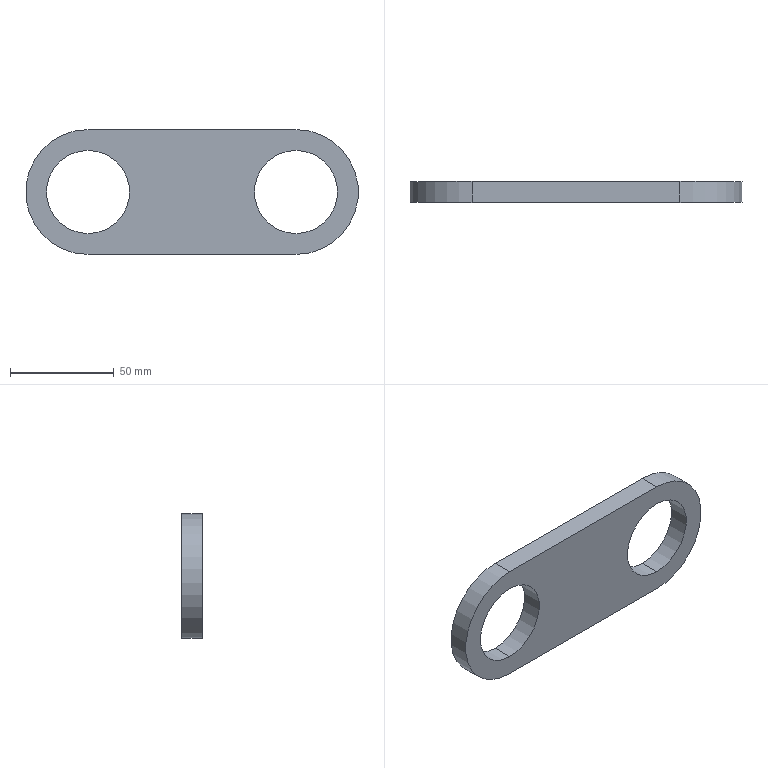Part | SolidWorks | features Extrusion 1 | 1 solid | 10 faces | box 160 x 10 x 60 mm | volume 63142 mm3 | cylinder 6 | plane 4 | commonest cylinder face diameters 40 x4 60 x2
STEP:
#1=CARTESIAN_POINT('',(-50.,10.,-20.));
#2=VERTEX_POINT('',#1);
#3=CARTESIAN_POINT('',(-50.,10.,20.));
#4=VERTEX_POINT('',#3);
#5=CARTESIAN_POINT('',(-50.,10.,0.));
#6=DIRECTION('',(0.,1.,0.));
#7=DIRECTION('',(0.,0.,1.));
#8=AXIS2_PLACEMENT_3D('',#5,#6,#7);
#9=CIRCLE('',#8,20.);
#10=EDGE_CURVE('',#2,#4,#9,.T.);
#11=ORIENTED_EDGE('',*,*,#10,.T.);
#12=CARTESIAN_POINT('',(-50.,0.,20.));
#13=VERTEX_POINT('',#12);
#14=CARTESIAN_POINT('',(-50.,10.,20.));
#15=DIRECTION('',(0.,-1.,0.));
#16=VECTOR('',#15,1000.);
#17=LINE('',#14,#16);
#18=EDGE_CURVE('',#4,#13,#17,.T.);
#19=ORIENTED_EDGE('',*,*,#18,.T.);
#20=CARTESIAN_POINT('',(-50.,0.,-20.));
#21=VERTEX_POINT('',#20);
#22=CARTESIAN_POINT('',(-50.,0.,0.));
#23=DIRECTION('',(0.,1.,0.));
#24=DIRECTION('',(0.,0.,1.));
#25=AXIS2_PLACEMENT_3D('',#22,#23,#24);
#26=CIRCLE('',#25,20.);
#27=EDGE_CURVE('',#21,#13,#26,.T.);
#28=ORIENTED_EDGE('',*,*,#27,.F.);
#29=CARTESIAN_POINT('',(-50.,10.,-20.));
#30=DIRECTION('',(0.,-1.,0.));
#31=VECTOR('',#30,1000.);
#32=LINE('',#29,#31);
#33=EDGE_CURVE('',#2,#21,#32,.T.);
#34=ORIENTED_EDGE('',*,*,#33,.F.);
#35=EDGE_LOOP('',(#11,#19,#28,#34));
#36=FACE_OUTER_BOUND('',#35,.T.);
#37=CARTESIAN_POINT('',(-50.,10.,0.));
#38=DIRECTION('',(0.,-1.,0.));
#39=DIRECTION('',(0.,0.,-1.));
#40=AXIS2_PLACEMENT_3D('',#37,#38,#39);
#41=CYLINDRICAL_SURFACE('',#40,20.);
#42=ADVANCED_FACE('',(#36),#41,.F.);
#43=CARTESIAN_POINT('',(50.,10.,-20.));
#44=VERTEX_POINT('',#43);
#45=CARTESIAN_POINT('',(50.,10.,20.));
#46=VERTEX_POINT('',#45);
#47=CARTESIAN_POINT('',(50.,10.,0.));
#48=DIRECTION('',(0.,1.,0.));
#49=DIRECTION('',(0.,0.,1.));
#50=AXIS2_PLACEMENT_3D('',#47,#48,#49);
#51=CIRCLE('',#50,20.);
#52=EDGE_CURVE('',#44,#46,#51,.T.);
#53=ORIENTED_EDGE('',*,*,#52,.T.);
#54=CARTESIAN_POINT('',(50.,0.,20.));
#55=VERTEX_POINT('',#54);
#56=CARTESIAN_POINT('',(50.,10.,20.));
#57=DIRECTION('',(0.,-1.,0.));
#58=VECTOR('',#57,1000.);
#59=LINE('',#56,#58);
#60=EDGE_CURVE('',#46,#55,#59,.T.);
#61=ORIENTED_EDGE('',*,*,#60,.T.);
#62=CARTESIAN_POINT('',(50.,0.,-20.));
#63=VERTEX_POINT('',#62);
#64=CARTESIAN_POINT('',(50.,0.,0.));
#65=DIRECTION('',(0.,1.,0.));
#66=DIRECTION('',(0.,0.,1.));
#67=AXIS2_PLACEMENT_3D('',#64,#65,#66);
#68=CIRCLE('',#67,20.);
#69=EDGE_CURVE('',#63,#55,#68,.T.);
#70=ORIENTED_EDGE('',*,*,#69,.F.);
#71=CARTESIAN_POINT('',(50.,10.,-20.));
#72=DIRECTION('',(0.,-1.,0.));
#73=VECTOR('',#72,1000.);
#74=LINE('',#71,#73);
#75=EDGE_CURVE('',#44,#63,#74,.T.);
#76=ORIENTED_EDGE('',*,*,#75,.F.);
#77=EDGE_LOOP('',(#53,#61,#70,#76));
#78=FACE_OUTER_BOUND('',#77,.T.);
#79=CARTESIAN_POINT('',(50.,10.,0.));
#80=DIRECTION('',(0.,-1.,0.));
#81=DIRECTION('',(0.,0.,-1.));
#82=AXIS2_PLACEMENT_3D('',#79,#80,#81);
#83=CYLINDRICAL_SURFACE('',#82,20.);
#84=ADVANCED_FACE('',(#78),#83,.F.);
#85=ORIENTED_EDGE('',*,*,#52,.F.);
#86=CARTESIAN_POINT('',(50.,10.,0.));
#87=DIRECTION('',(0.,1.,0.));
#88=DIRECTION('',(0.,0.,1.));
#89=AXIS2_PLACEMENT_3D('',#86,#87,#88);
#90=CIRCLE('',#89,20.);
#91=EDGE_CURVE('',#46,#44,#90,.T.);
#92=ORIENTED_EDGE('',*,*,#91,.F.);
#93=EDGE_LOOP('',(#85,#92));
#94=FACE_BOUND('',#93,.T.);
#95=CARTESIAN_POINT('',(-50.,10.,-30.));
#96=VERTEX_POINT('',#95);
#97=CARTESIAN_POINT('',(-50.,10.,30.));
#98=VERTEX_POINT('',#97);
#99=CARTESIAN_POINT('',(-50.,10.,0.));
#100=DIRECTION('',(0.,1.,0.));
#101=DIRECTION('',(0.,0.,1.));
#102=AXIS2_PLACEMENT_3D('',#99,#100,#101);
#103=CIRCLE('',#102,30.);
#104=EDGE_CURVE('',#96,#98,#103,.T.);
#105=ORIENTED_EDGE('',*,*,#104,.T.);
#106=CARTESIAN_POINT('',(50.,10.,30.));
#107=VERTEX_POINT('',#106);
#108=CARTESIAN_POINT('',(-50.,10.,30.));
#109=DIRECTION('',(1.,0.,0.));
#110=VECTOR('',#109,1000.);
#111=LINE('',#108,#110);
#112=EDGE_CURVE('',#98,#107,#111,.T.);
#113=ORIENTED_EDGE('',*,*,#112,.T.);
#114=CARTESIAN_POINT('',(50.,10.,-30.));
#115=VERTEX_POINT('',#114);
#116=CARTESIAN_POINT('',(50.,10.,0.));
#117=DIRECTION('',(0.,1.,0.));
#118=DIRECTION('',(0.,0.,1.));
#119=AXIS2_PLACEMENT_3D('',#116,#117,#118);
#120=CIRCLE('',#119,30.);
#121=EDGE_CURVE('',#107,#115,#120,.T.);
#122=ORIENTED_EDGE('',*,*,#121,.T.);
#123=CARTESIAN_POINT('',(-50.,10.,-30.));
#124=DIRECTION('',(-1.,0.,0.));
#125=VECTOR('',#124,1000.);
#126=LINE('',#123,#125);
#127=EDGE_CURVE('',#115,#96,#126,.T.);
#128=ORIENTED_EDGE('',*,*,#127,.T.);
#129=EDGE_LOOP('',(#105,#113,#122,#128));
#130=FACE_OUTER_BOUND('',#129,.T.);
#131=ORIENTED_EDGE('',*,*,#10,.F.);
#132=CARTESIAN_POINT('',(-50.,10.,0.));
#133=DIRECTION('',(0.,1.,0.));
#134=DIRECTION('',(0.,0.,1.));
#135=AXIS2_PLACEMENT_3D('',#132,#133,#134);
#136=CIRCLE('',#135,20.);
#137=EDGE_CURVE('',#4,#2,#136,.T.);
#138=ORIENTED_EDGE('',*,*,#137,.F.);
#139=EDGE_LOOP('',(#131,#138));
#140=FACE_BOUND('',#139,.T.);
#141=CARTESIAN_POINT('',(-50.,10.,0.));
#142=DIRECTION('',(0.,1.,0.));
#143=DIRECTION('',(0.,0.,1.));
#144=AXIS2_PLACEMENT_3D('',#141,#142,#143);
#145=PLANE('',#144);
#146=ADVANCED_FACE('',(#94,#130,#140),#145,.T.);
#147=CARTESIAN_POINT('',(-50.,0.,-30.));
#148=VERTEX_POINT('',#147);
#149=CARTESIAN_POINT('',(-50.,0.,30.));
#150=VERTEX_POINT('',#149);
#151=CARTESIAN_POINT('',(-50.,0.,0.));
#152=DIRECTION('',(0.,1.,0.));
#153=DIRECTION('',(0.,0.,1.));
#154=AXIS2_PLACEMENT_3D('',#151,#152,#153);
#155=CIRCLE('',#154,30.);
#156=EDGE_CURVE('',#148,#150,#155,.T.);
#157=ORIENTED_EDGE('',*,*,#156,.F.);
#158=CARTESIAN_POINT('',(50.,0.,-30.));
#159=VERTEX_POINT('',#158);
#160=CARTESIAN_POINT('',(-50.,0.,-30.));
#161=DIRECTION('',(-1.,0.,0.));
#162=VECTOR('',#161,1000.);
#163=LINE('',#160,#162);
#164=EDGE_CURVE('',#159,#148,#163,.T.);
#165=ORIENTED_EDGE('',*,*,#164,.F.);
#166=CARTESIAN_POINT('',(50.,0.,30.));
#167=VERTEX_POINT('',#166);
#168=CARTESIAN_POINT('',(50.,0.,0.));
#169=DIRECTION('',(0.,1.,0.));
#170=DIRECTION('',(0.,0.,1.));
#171=AXIS2_PLACEMENT_3D('',#168,#169,#170);
#172=CIRCLE('',#171,30.);
#173=EDGE_CURVE('',#167,#159,#172,.T.);
#174=ORIENTED_EDGE('',*,*,#173,.F.);
#175=CARTESIAN_POINT('',(-50.,0.,30.));
#176=DIRECTION('',(1.,0.,0.));
#177=VECTOR('',#176,1000.);
#178=LINE('',#175,#177);
#179=EDGE_CURVE('',#150,#167,#178,.T.);
#180=ORIENTED_EDGE('',*,*,#179,.F.);
#181=EDGE_LOOP('',(#157,#165,#174,#180));
#182=FACE_OUTER_BOUND('',#181,.T.);
#183=ORIENTED_EDGE('',*,*,#69,.T.);
#184=CARTESIAN_POINT('',(50.,0.,0.));
#185=DIRECTION('',(0.,1.,0.));
#186=DIRECTION('',(0.,0.,1.));
#187=AXIS2_PLACEMENT_3D('',#184,#185,#186);
#188=CIRCLE('',#187,20.);
#189=EDGE_CURVE('',#55,#63,#188,.T.);
#190=ORIENTED_EDGE('',*,*,#189,.T.);
#191=EDGE_LOOP('',(#183,#190));
#192=FACE_BOUND('',#191,.T.);
#193=ORIENTED_EDGE('',*,*,#27,.T.);
#194=CARTESIAN_POINT('',(-50.,0.,0.));
#195=DIRECTION('',(0.,1.,0.));
#196=DIRECTION('',(0.,0.,1.));
#197=AXIS2_PLACEMENT_3D('',#194,#195,#196);
#198=CIRCLE('',#197,20.);
#199=EDGE_CURVE('',#13,#21,#198,.T.);
#200=ORIENTED_EDGE('',*,*,#199,.T.);
#201=EDGE_LOOP('',(#193,#200));
#202=FACE_BOUND('',#201,.T.);
#203=CARTESIAN_POINT('',(-50.,0.,0.));
#204=DIRECTION('',(0.,1.,0.));
#205=DIRECTION('',(0.,0.,1.));
#206=AXIS2_PLACEMENT_3D('',#203,#204,#205);
#207=PLANE('',#206);
#208=ADVANCED_FACE('',(#182,#192,#202),#207,.F.);
#209=ORIENTED_EDGE('',*,*,#156,.T.);
#210=CARTESIAN_POINT('',(-50.,10.,30.));
#211=DIRECTION('',(0.,-1.,0.));
#212=VECTOR('',#211,1000.);
#213=LINE('',#210,#212);
#214=EDGE_CURVE('',#98,#150,#213,.T.);
#215=ORIENTED_EDGE('',*,*,#214,.F.);
#216=ORIENTED_EDGE('',*,*,#104,.F.);
#217=CARTESIAN_POINT('',(-50.,10.,-30.));
#218=DIRECTION('',(0.,-1.,0.));
#219=VECTOR('',#218,1000.);
#220=LINE('',#217,#219);
#221=EDGE_CURVE('',#96,#148,#220,.T.);
#222=ORIENTED_EDGE('',*,*,#221,.T.);
#223=EDGE_LOOP('',(#209,#215,#216,#222));
#224=FACE_OUTER_BOUND('',#223,.T.);
#225=CARTESIAN_POINT('',(-50.,10.,0.));
#226=DIRECTION('',(0.,-1.,0.));
#227=DIRECTION('',(0.,0.,-1.));
#228=AXIS2_PLACEMENT_3D('',#225,#226,#227);
#229=CYLINDRICAL_SURFACE('',#228,30.);
#230=ADVANCED_FACE('',(#224),#229,.T.);
#231=ORIENTED_EDGE('',*,*,#179,.T.);
#232=CARTESIAN_POINT('',(50.,10.,30.));
#233=DIRECTION('',(0.,-1.,0.));
#234=VECTOR('',#233,1000.);
#235=LINE('',#232,#234);
#236=EDGE_CURVE('',#107,#167,#235,.T.);
#237=ORIENTED_EDGE('',*,*,#236,.F.);
#238=ORIENTED_EDGE('',*,*,#112,.F.);
#239=ORIENTED_EDGE('',*,*,#214,.T.);
#240=EDGE_LOOP('',(#231,#237,#238,#239));
#241=FACE_OUTER_BOUND('',#240,.T.);
#242=CARTESIAN_POINT('',(-50.,10.,30.));
#243=DIRECTION('',(0.,0.,-1.));
#244=DIRECTION('',(-1.,0.,0.));
#245=AXIS2_PLACEMENT_3D('',#242,#243,#244);
#246=PLANE('',#245);
#247=ADVANCED_FACE('',(#241),#246,.F.);
#248=ORIENTED_EDGE('',*,*,#173,.T.);
#249=CARTESIAN_POINT('',(50.,10.,-30.));
#250=DIRECTION('',(0.,-1.,0.));
#251=VECTOR('',#250,1000.);
#252=LINE('',#249,#251);
#253=EDGE_CURVE('',#115,#159,#252,.T.);
#254=ORIENTED_EDGE('',*,*,#253,.F.);
#255=ORIENTED_EDGE('',*,*,#121,.F.);
#256=ORIENTED_EDGE('',*,*,#236,.T.);
#257=EDGE_LOOP('',(#248,#254,#255,#256));
#258=FACE_OUTER_BOUND('',#257,.T.);
#259=CARTESIAN_POINT('',(50.,10.,0.));
#260=DIRECTION('',(0.,-1.,0.));
#261=DIRECTION('',(0.,0.,-1.));
#262=AXIS2_PLACEMENT_3D('',#259,#260,#261);
#263=CYLINDRICAL_SURFACE('',#262,30.);
#264=ADVANCED_FACE('',(#258),#263,.T.);
#265=ORIENTED_EDGE('',*,*,#164,.T.);
#266=ORIENTED_EDGE('',*,*,#221,.F.);
#267=ORIENTED_EDGE('',*,*,#127,.F.);
#268=ORIENTED_EDGE('',*,*,#253,.T.);
#269=EDGE_LOOP('',(#265,#266,#267,#268));
#270=FACE_OUTER_BOUND('',#269,.T.);
#271=CARTESIAN_POINT('',(-50.,10.,-30.));
#272=DIRECTION('',(0.,0.,1.));
#273=DIRECTION('',(1.,0.,0.));
#274=AXIS2_PLACEMENT_3D('',#271,#272,#273);
#275=PLANE('',#274);
#276=ADVANCED_FACE('',(#270),#275,.F.);
#277=ORIENTED_EDGE('',*,*,#60,.F.);
#278=ORIENTED_EDGE('',*,*,#91,.T.);
#279=ORIENTED_EDGE('',*,*,#75,.T.);
#280=ORIENTED_EDGE('',*,*,#189,.F.);
#281=EDGE_LOOP('',(#277,#278,#279,#280));
#282=FACE_OUTER_BOUND('',#281,.T.);
#283=CARTESIAN_POINT('',(50.,10.,0.));
#284=DIRECTION('',(0.,-1.,0.));
#285=DIRECTION('',(0.,0.,-1.));
#286=AXIS2_PLACEMENT_3D('',#283,#284,#285);
#287=CYLINDRICAL_SURFACE('',#286,20.);
#288=ADVANCED_FACE('',(#282),#287,.F.);
#289=ORIENTED_EDGE('',*,*,#18,.F.);
#290=ORIENTED_EDGE('',*,*,#137,.T.);
#291=ORIENTED_EDGE('',*,*,#33,.T.);
#292=ORIENTED_EDGE('',*,*,#199,.F.);
#293=EDGE_LOOP('',(#289,#290,#291,#292));
#294=FACE_OUTER_BOUND('',#293,.T.);
#295=CARTESIAN_POINT('',(-50.,10.,0.));
#296=DIRECTION('',(0.,-1.,0.));
#297=DIRECTION('',(0.,0.,-1.));
#298=AXIS2_PLACEMENT_3D('',#295,#296,#297);
#299=CYLINDRICAL_SURFACE('',#298,20.);
#300=ADVANCED_FACE('',(#294),#299,.F.);
#301=CLOSED_SHELL('',(#42,#84,#146,#208,#230,#247,#264,#276,#288,#300));
#302=MANIFOLD_SOLID_BREP('',#301);
#303=CARTESIAN_POINT('',(0.,0.,0.));
#304=DIRECTION('',(0.,0.,1.));
#305=DIRECTION('',(1.,0.,0.));
#306=AXIS2_PLACEMENT_3D('',#303,#304,#305);
#307=(LENGTH_UNIT()NAMED_UNIT(*)SI_UNIT(.MILLI.,.METRE.));
#308=UNCERTAINTY_MEASURE_WITH_UNIT(LENGTH_MEASURE(0.00001),#307,'','');
#309=(NAMED_UNIT(*)PLANE_ANGLE_UNIT()SI_UNIT($,.RADIAN.));
#310=(NAMED_UNIT(*)SI_UNIT($,.STERADIAN.)SOLID_ANGLE_UNIT());
#311=(GEOMETRIC_REPRESENTATION_CONTEXT(3)GLOBAL_UNCERTAINTY_ASSIGNED_CONTEXT((#308))GLOBAL_UNIT_ASSIGNED_CONTEXT((#307,#309,#310))REPRESENTATION_CONTEXT('',''));
#312=ADVANCED_BREP_SHAPE_REPRESENTATION('',(#302,#306),#311);